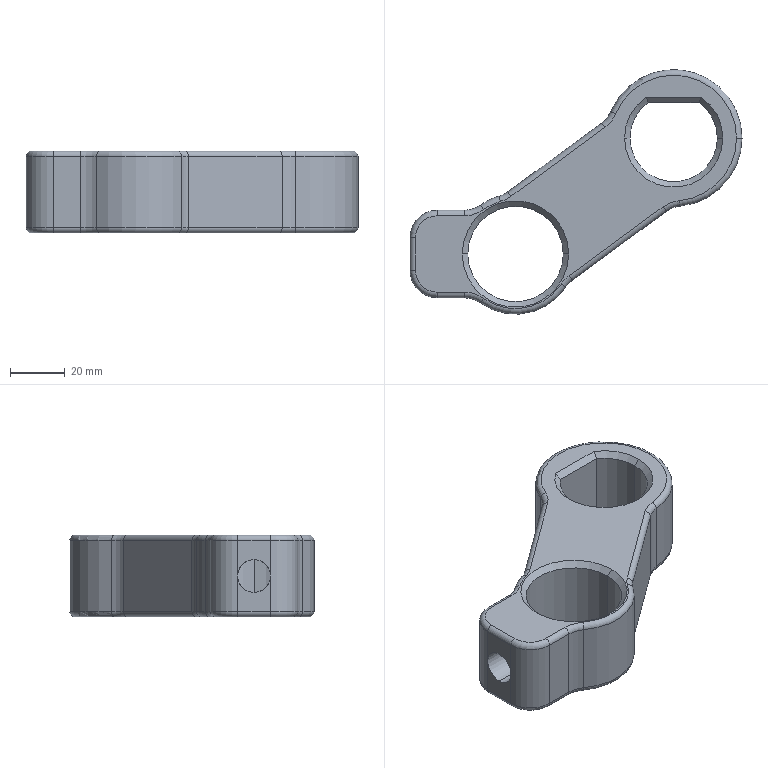Part | SolidWorks | features Fillet 2, Chamfer 1, Extrusion 1, ICE 1 | 1 solid | 73 faces | box 121.493 x 89.432 x 30 mm | volume 103342 mm3 | cylinder 28 | torus 24 | plane 11 | cone 10 | commonest cylinder face diameters 4 x10 20 x8 32 x3 12 x2 35 x2 44 x2